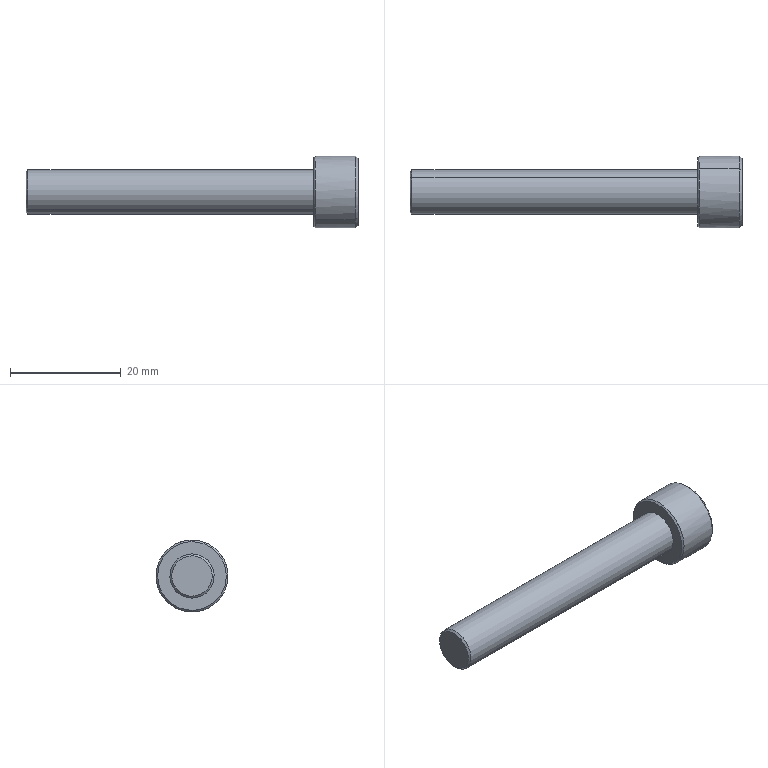Part | STEP file | BOLT(all)(M8X60) | 1 solid | 20 faces | box 60 x 13 x 13 mm | volume 3384 mm3 | plane 10 | cone 6 | cylinder 4 | commonest cylinder face diameters 8 x2 13 x2